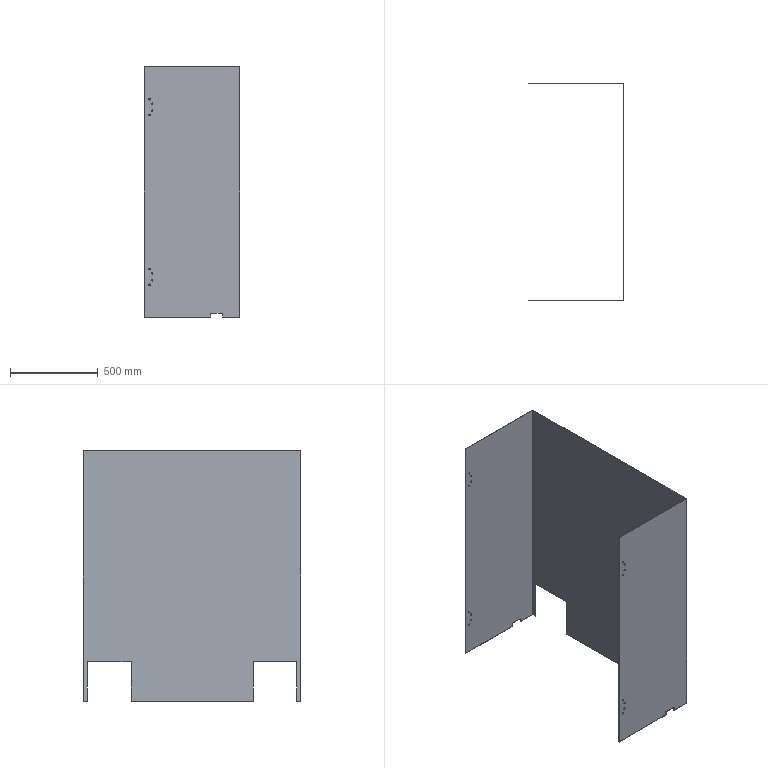Part | SolidWorks | features BaseBody 1 | 1 solid | 58 faces | box 544 x 1240 x 1428 mm | volume 6405923 mm3 | cylinder 32 | plane 26 | commonest cylinder face diameters 8.5 x32